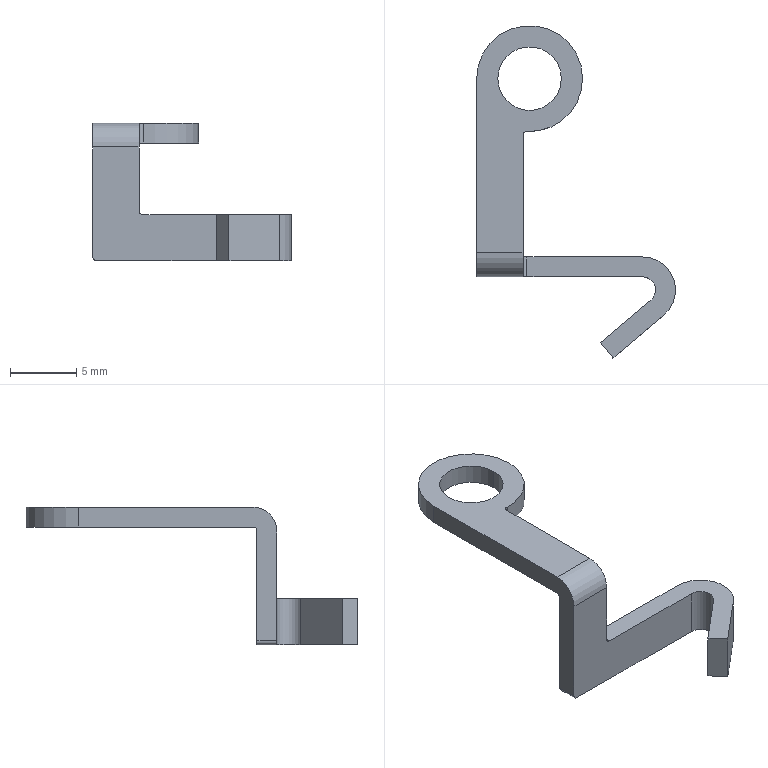Part | STEP file | TQ-DD-1105-THTerminalD1010_デフォルト | 1 solid | 22 faces | box 15.02 x 25.091 x 10.4 mm | volume 251.396 mm3 | cylinder 11 | plane 11 | commonest cylinder face diameters 0.6 x4 4.8 x2 8 x2 2 x1 3.6 x1 5 x1
STEP:
#1=CARTESIAN_POINT('',(2.4,0.,0.));
#2=VERTEX_POINT('',#1);
#3=CARTESIAN_POINT('',(-2.4,0.,0.));
#4=VERTEX_POINT('',#3);
#5=CARTESIAN_POINT('',(0.,0.,0.));
#6=DIRECTION('',(0.,0.,-1.));
#7=DIRECTION('',(1.,0.,0.));
#8=AXIS2_PLACEMENT_3D('',#5,#6,#7);
#9=CIRCLE('',#8,2.4);
#10=EDGE_CURVE('',#2,#4,#9,.T.);
#11=ORIENTED_EDGE('',*,*,#10,.T.);
#12=CARTESIAN_POINT('',(-2.4,0.,1.5));
#13=VERTEX_POINT('',#12);
#14=CARTESIAN_POINT('',(-2.4,0.,0.75));
#15=DIRECTION('',(0.,0.,1.));
#16=VECTOR('',#15,1000.);
#17=LINE('',#14,#16);
#18=EDGE_CURVE('',#4,#13,#17,.T.);
#19=ORIENTED_EDGE('',*,*,#18,.T.);
#20=CARTESIAN_POINT('',(2.4,0.,1.5));
#21=VERTEX_POINT('',#20);
#22=CARTESIAN_POINT('',(0.,0.,1.5));
#23=DIRECTION('',(0.,0.,-1.));
#24=DIRECTION('',(1.,0.,0.));
#25=AXIS2_PLACEMENT_3D('',#22,#23,#24);
#26=CIRCLE('',#25,2.4);
#27=EDGE_CURVE('',#21,#13,#26,.T.);
#28=ORIENTED_EDGE('',*,*,#27,.F.);
#29=CARTESIAN_POINT('',(2.4,0.,0.75));
#30=DIRECTION('',(0.,0.,1.));
#31=VECTOR('',#30,1000.);
#32=LINE('',#29,#31);
#33=EDGE_CURVE('',#2,#21,#32,.T.);
#34=ORIENTED_EDGE('',*,*,#33,.F.);
#35=EDGE_LOOP('',(#11,#19,#28,#34));
#36=FACE_OUTER_BOUND('',#35,.T.);
#37=CARTESIAN_POINT('',(0.,0.,0.75));
#38=DIRECTION('',(0.,0.,1.));
#39=DIRECTION('',(1.,0.,0.));
#40=AXIS2_PLACEMENT_3D('',#37,#38,#39);
#41=CYLINDRICAL_SURFACE('',#40,2.4);
#42=ADVANCED_FACE('',(#36),#41,.F.);
#43=CARTESIAN_POINT('',(-0.186,-3.996,0.));
#44=VERTEX_POINT('',#43);
#45=CARTESIAN_POINT('',(4.,0.,0.));
#46=VERTEX_POINT('',#45);
#47=CARTESIAN_POINT('',(0.,0.,0.));
#48=DIRECTION('',(0.,0.,1.));
#49=DIRECTION('',(1.,0.,0.));
#50=AXIS2_PLACEMENT_3D('',#47,#48,#49);
#51=CIRCLE('',#50,4.);
#52=EDGE_CURVE('',#44,#46,#51,.T.);
#53=ORIENTED_EDGE('',*,*,#52,.T.);
#54=CARTESIAN_POINT('',(4.,0.,1.5));
#55=VERTEX_POINT('',#54);
#56=CARTESIAN_POINT('',(4.,0.,0.75));
#57=DIRECTION('',(0.,0.,1.));
#58=VECTOR('',#57,1000.);
#59=LINE('',#56,#58);
#60=EDGE_CURVE('',#46,#55,#59,.T.);
#61=ORIENTED_EDGE('',*,*,#60,.T.);
#62=CARTESIAN_POINT('',(-0.186,-3.996,1.5));
#63=VERTEX_POINT('',#62);
#64=CARTESIAN_POINT('',(0.,0.,1.5));
#65=DIRECTION('',(0.,0.,-1.));
#66=DIRECTION('',(1.,0.,0.));
#67=AXIS2_PLACEMENT_3D('',#64,#65,#66);
#68=CIRCLE('',#67,4.);
#69=EDGE_CURVE('',#55,#63,#68,.T.);
#70=ORIENTED_EDGE('',*,*,#69,.T.);
#71=CARTESIAN_POINT('',(-0.186,-3.996,0.75));
#72=DIRECTION('',(0.,0.,-1.));
#73=VECTOR('',#72,1000.);
#74=LINE('',#71,#73);
#75=EDGE_CURVE('',#63,#44,#74,.T.);
#76=ORIENTED_EDGE('',*,*,#75,.T.);
#77=EDGE_LOOP('',(#53,#61,#70,#76));
#78=FACE_OUTER_BOUND('',#77,.T.);
#79=CARTESIAN_POINT('',(0.,0.,0.75));
#80=DIRECTION('',(0.,0.,1.));
#81=DIRECTION('',(1.,0.,0.));
#82=AXIS2_PLACEMENT_3D('',#79,#80,#81);
#83=CYLINDRICAL_SURFACE('',#82,4.);
#84=ADVANCED_FACE('',(#78),#83,.T.);
#85=ORIENTED_EDGE('',*,*,#10,.F.);
#86=CARTESIAN_POINT('',(0.,0.,0.));
#87=DIRECTION('',(0.,0.,-1.));
#88=DIRECTION('',(1.,0.,0.));
#89=AXIS2_PLACEMENT_3D('',#86,#87,#88);
#90=CIRCLE('',#89,2.4);
#91=EDGE_CURVE('',#4,#2,#90,.T.);
#92=ORIENTED_EDGE('',*,*,#91,.F.);
#93=EDGE_LOOP('',(#85,#92));
#94=FACE_BOUND('',#93,.T.);
#95=CARTESIAN_POINT('',(-4.,0.,0.));
#96=VERTEX_POINT('',#95);
#97=CARTESIAN_POINT('',(-4.,-13.162,0.));
#98=VERTEX_POINT('',#97);
#99=CARTESIAN_POINT('',(-4.,0.,0.));
#100=DIRECTION('',(0.,-1.,0.));
#101=VECTOR('',#100,1000.);
#102=LINE('',#99,#101);
#103=EDGE_CURVE('',#96,#98,#102,.T.);
#104=ORIENTED_EDGE('',*,*,#103,.F.);
#105=CARTESIAN_POINT('',(0.,0.,0.));
#106=DIRECTION('',(0.,0.,1.));
#107=DIRECTION('',(1.,0.,0.));
#108=AXIS2_PLACEMENT_3D('',#105,#106,#107);
#109=CIRCLE('',#108,4.);
#110=EDGE_CURVE('',#46,#96,#109,.T.);
#111=ORIENTED_EDGE('',*,*,#110,.F.);
#112=ORIENTED_EDGE('',*,*,#52,.F.);
#113=CARTESIAN_POINT('',(-0.5,-4.295,0.));
#114=VERTEX_POINT('',#113);
#115=CARTESIAN_POINT('',(-0.2,-4.295,0.));
#116=DIRECTION('',(0.,0.,1.));
#117=DIRECTION('',(1.,0.,0.));
#118=AXIS2_PLACEMENT_3D('',#115,#116,#117);
#119=CIRCLE('',#118,0.3);
#120=EDGE_CURVE('',#44,#114,#119,.T.);
#121=ORIENTED_EDGE('',*,*,#120,.T.);
#122=CARTESIAN_POINT('',(-0.5,-13.162,0.));
#123=VERTEX_POINT('',#122);
#124=CARTESIAN_POINT('',(-0.5,0.,0.));
#125=DIRECTION('',(0.,1.,0.));
#126=VECTOR('',#125,1000.);
#127=LINE('',#124,#126);
#128=EDGE_CURVE('',#123,#114,#127,.T.);
#129=ORIENTED_EDGE('',*,*,#128,.F.);
#130=CARTESIAN_POINT('',(0.,-13.162,0.));
#131=DIRECTION('',(1.,0.,0.));
#132=VECTOR('',#131,1000.);
#133=LINE('',#130,#132);
#134=EDGE_CURVE('',#98,#123,#133,.T.);
#135=ORIENTED_EDGE('',*,*,#134,.F.);
#136=EDGE_LOOP('',(#104,#111,#112,#121,#129,#135));
#137=FACE_OUTER_BOUND('',#136,.T.);
#138=CARTESIAN_POINT('',(0.,0.,0.));
#139=DIRECTION('',(0.,0.,1.));
#140=DIRECTION('',(1.,0.,0.));
#141=AXIS2_PLACEMENT_3D('',#138,#139,#140);
#142=PLANE('',#141);
#143=ADVANCED_FACE('',(#94,#137),#142,.F.);
#144=ORIENTED_EDGE('',*,*,#18,.F.);
#145=ORIENTED_EDGE('',*,*,#91,.T.);
#146=ORIENTED_EDGE('',*,*,#33,.T.);
#147=CARTESIAN_POINT('',(0.,0.,1.5));
#148=DIRECTION('',(0.,0.,-1.));
#149=DIRECTION('',(1.,0.,0.));
#150=AXIS2_PLACEMENT_3D('',#147,#148,#149);
#151=CIRCLE('',#150,2.4);
#152=EDGE_CURVE('',#13,#21,#151,.T.);
#153=ORIENTED_EDGE('',*,*,#152,.F.);
#154=EDGE_LOOP('',(#144,#145,#146,#153));
#155=FACE_OUTER_BOUND('',#154,.T.);
#156=CARTESIAN_POINT('',(0.,0.,0.75));
#157=DIRECTION('',(0.,0.,1.));
#158=DIRECTION('',(1.,0.,0.));
#159=AXIS2_PLACEMENT_3D('',#156,#157,#158);
#160=CYLINDRICAL_SURFACE('',#159,2.4);
#161=ADVANCED_FACE('',(#155),#160,.F.);
#162=CARTESIAN_POINT('',(-0.5,-13.462,-0.3));
#163=VERTEX_POINT('',#162);
#164=CARTESIAN_POINT('',(-0.5,-13.162,-0.3));
#165=DIRECTION('',(-1.,0.,0.));
#166=DIRECTION('',(0.,0.,-1.));
#167=AXIS2_PLACEMENT_3D('',#164,#165,#166);
#168=CIRCLE('',#167,0.3);
#169=EDGE_CURVE('',#163,#123,#168,.T.);
#170=ORIENTED_EDGE('',*,*,#169,.F.);
#171=CARTESIAN_POINT('',(-4.,-13.462,-0.3));
#172=VERTEX_POINT('',#171);
#173=CARTESIAN_POINT('',(0.,-13.462,-0.3));
#174=DIRECTION('',(1.,0.,0.));
#175=VECTOR('',#174,1000.);
#176=LINE('',#173,#175);
#177=EDGE_CURVE('',#172,#163,#176,.T.);
#178=ORIENTED_EDGE('',*,*,#177,.F.);
#179=CARTESIAN_POINT('',(-4.,-13.162,-0.3));
#180=DIRECTION('',(1.,0.,0.));
#181=DIRECTION('',(0.,0.,-1.));
#182=AXIS2_PLACEMENT_3D('',#179,#180,#181);
#183=CIRCLE('',#182,0.3);
#184=EDGE_CURVE('',#98,#172,#183,.T.);
#185=ORIENTED_EDGE('',*,*,#184,.F.);
#186=ORIENTED_EDGE('',*,*,#134,.T.);
#187=EDGE_LOOP('',(#170,#178,#185,#186));
#188=FACE_OUTER_BOUND('',#187,.T.);
#189=CARTESIAN_POINT('',(0.,-13.162,-0.3));
#190=DIRECTION('',(1.,0.,0.));
#191=DIRECTION('',(0.,0.,-1.));
#192=AXIS2_PLACEMENT_3D('',#189,#190,#191);
#193=CYLINDRICAL_SURFACE('',#192,0.3);
#194=ADVANCED_FACE('',(#188),#193,.F.);
#195=CARTESIAN_POINT('',(-4.,-13.462,-8.6));
#196=VERTEX_POINT('',#195);
#197=CARTESIAN_POINT('',(-4.,-13.462,0.));
#198=DIRECTION('',(0.,0.,-1.));
#199=VECTOR('',#198,1000.);
#200=LINE('',#197,#199);
#201=EDGE_CURVE('',#172,#196,#200,.T.);
#202=ORIENTED_EDGE('',*,*,#201,.T.);
#203=CARTESIAN_POINT('',(-4.,-14.962,-8.6));
#204=VERTEX_POINT('',#203);
#205=CARTESIAN_POINT('',(-4.,0.,-8.6));
#206=DIRECTION('',(0.,-1.,0.));
#207=VECTOR('',#206,1000.);
#208=LINE('',#205,#207);
#209=EDGE_CURVE('',#196,#204,#208,.T.);
#210=ORIENTED_EDGE('',*,*,#209,.T.);
#211=CARTESIAN_POINT('',(-4.,-14.962,-0.3));
#212=VERTEX_POINT('',#211);
#213=CARTESIAN_POINT('',(-4.,-14.962,0.));
#214=DIRECTION('',(0.,0.,1.));
#215=VECTOR('',#214,1000.);
#216=LINE('',#213,#215);
#217=EDGE_CURVE('',#204,#212,#216,.T.);
#218=ORIENTED_EDGE('',*,*,#217,.T.);
#219=CARTESIAN_POINT('',(-4.,-13.162,1.5));
#220=VERTEX_POINT('',#219);
#221=CARTESIAN_POINT('',(-4.,-13.162,-0.3));
#222=DIRECTION('',(-1.,0.,0.));
#223=DIRECTION('',(0.,0.,1.));
#224=AXIS2_PLACEMENT_3D('',#221,#222,#223);
#225=CIRCLE('',#224,1.8);
#226=EDGE_CURVE('',#212,#220,#225,.T.);
#227=ORIENTED_EDGE('',*,*,#226,.T.);
#228=CARTESIAN_POINT('',(-4.,0.,1.5));
#229=VERTEX_POINT('',#228);
#230=CARTESIAN_POINT('',(-4.,0.,1.5));
#231=DIRECTION('',(0.,1.,0.));
#232=VECTOR('',#231,1000.);
#233=LINE('',#230,#232);
#234=EDGE_CURVE('',#220,#229,#233,.T.);
#235=ORIENTED_EDGE('',*,*,#234,.T.);
#236=CARTESIAN_POINT('',(-4.,0.,0.));
#237=DIRECTION('',(0.,0.,-1.));
#238=VECTOR('',#237,1000.);
#239=LINE('',#236,#238);
#240=EDGE_CURVE('',#229,#96,#239,.T.);
#241=ORIENTED_EDGE('',*,*,#240,.T.);
#242=ORIENTED_EDGE('',*,*,#103,.T.);
#243=ORIENTED_EDGE('',*,*,#184,.T.);
#244=EDGE_LOOP('',(#202,#210,#218,#227,#235,#241,#242,#243));
#245=FACE_OUTER_BOUND('',#244,.T.);
#246=CARTESIAN_POINT('',(-4.,0.,0.));
#247=DIRECTION('',(-1.,0.,0.));
#248=DIRECTION('',(0.,0.,1.));
#249=AXIS2_PLACEMENT_3D('',#246,#247,#248);
#250=PLANE('',#249);
#251=ADVANCED_FACE('',(#245),#250,.T.);
#252=ORIENTED_EDGE('',*,*,#60,.F.);
#253=ORIENTED_EDGE('',*,*,#110,.T.);
#254=ORIENTED_EDGE('',*,*,#240,.F.);
#255=CARTESIAN_POINT('',(0.,0.,1.5));
#256=DIRECTION('',(0.,0.,-1.));
#257=DIRECTION('',(1.,0.,0.));
#258=AXIS2_PLACEMENT_3D('',#255,#256,#257);
#259=CIRCLE('',#258,4.);
#260=EDGE_CURVE('',#229,#55,#259,.T.);
#261=ORIENTED_EDGE('',*,*,#260,.T.);
#262=EDGE_LOOP('',(#252,#253,#254,#261));
#263=FACE_OUTER_BOUND('',#262,.T.);
#264=CARTESIAN_POINT('',(0.,0.,0.75));
#265=DIRECTION('',(0.,0.,1.));
#266=DIRECTION('',(1.,0.,0.));
#267=AXIS2_PLACEMENT_3D('',#264,#265,#266);
#268=CYLINDRICAL_SURFACE('',#267,4.);
#269=ADVANCED_FACE('',(#263),#268,.T.);
#270=CARTESIAN_POINT('',(-0.5,-14.962,-0.3));
#271=VERTEX_POINT('',#270);
#272=CARTESIAN_POINT('',(-0.5,-14.962,-5.1));
#273=VERTEX_POINT('',#272);
#274=CARTESIAN_POINT('',(-0.5,-14.962,0.));
#275=DIRECTION('',(0.,0.,-1.));
#276=VECTOR('',#275,1000.);
#277=LINE('',#274,#276);
#278=EDGE_CURVE('',#271,#273,#277,.T.);
#279=ORIENTED_EDGE('',*,*,#278,.T.);
#280=CARTESIAN_POINT('',(-0.5,-13.462,-5.1));
#281=VERTEX_POINT('',#280);
#282=CARTESIAN_POINT('',(-0.5,-14.962,-5.1));
#283=DIRECTION('',(0.,1.,0.));
#284=VECTOR('',#283,1000.);
#285=LINE('',#282,#284);
#286=EDGE_CURVE('',#273,#281,#285,.T.);
#287=ORIENTED_EDGE('',*,*,#286,.T.);
#288=CARTESIAN_POINT('',(-0.5,-13.462,0.));
#289=DIRECTION('',(0.,0.,1.));
#290=VECTOR('',#289,1000.);
#291=LINE('',#288,#290);
#292=EDGE_CURVE('',#281,#163,#291,.T.);
#293=ORIENTED_EDGE('',*,*,#292,.T.);
#294=ORIENTED_EDGE('',*,*,#169,.T.);
#295=ORIENTED_EDGE('',*,*,#128,.T.);
#296=CARTESIAN_POINT('',(-0.5,-4.295,1.5));
#297=VERTEX_POINT('',#296);
#298=CARTESIAN_POINT('',(-0.5,-4.295,0.));
#299=DIRECTION('',(0.,0.,1.));
#300=VECTOR('',#299,1000.);
#301=LINE('',#298,#300);
#302=EDGE_CURVE('',#114,#297,#301,.T.);
#303=ORIENTED_EDGE('',*,*,#302,.T.);
#304=CARTESIAN_POINT('',(-0.5,-13.162,1.5));
#305=VERTEX_POINT('',#304);
#306=CARTESIAN_POINT('',(-0.5,-14.962,1.5));
#307=DIRECTION('',(0.,-1.,0.));
#308=VECTOR('',#307,1000.);
#309=LINE('',#306,#308);
#310=EDGE_CURVE('',#297,#305,#309,.T.);
#311=ORIENTED_EDGE('',*,*,#310,.T.);
#312=CARTESIAN_POINT('',(-0.5,-13.162,-0.3));
#313=DIRECTION('',(1.,0.,0.));
#314=DIRECTION('',(0.,0.,1.));
#315=AXIS2_PLACEMENT_3D('',#312,#313,#314);
#316=CIRCLE('',#315,1.8);
#317=EDGE_CURVE('',#305,#271,#316,.T.);
#318=ORIENTED_EDGE('',*,*,#317,.T.);
#319=EDGE_LOOP('',(#279,#287,#293,#294,#295,#303,#311,#318));
#320=FACE_OUTER_BOUND('',#319,.T.);
#321=CARTESIAN_POINT('',(-0.5,-14.962,0.));
#322=DIRECTION('',(1.,0.,0.));
#323=DIRECTION('',(0.,0.,-1.));
#324=AXIS2_PLACEMENT_3D('',#321,#322,#323);
#325=PLANE('',#324);
#326=ADVANCED_FACE('',(#320),#325,.T.);
#327=ORIENTED_EDGE('',*,*,#27,.T.);
#328=ORIENTED_EDGE('',*,*,#152,.T.);
#329=EDGE_LOOP('',(#327,#328));
#330=FACE_BOUND('',#329,.T.);
#331=ORIENTED_EDGE('',*,*,#234,.F.);
#332=CARTESIAN_POINT('',(0.,-13.162,1.5));
#333=DIRECTION('',(1.,0.,0.));
#334=VECTOR('',#333,1000.);
#335=LINE('',#332,#334);
#336=EDGE_CURVE('',#220,#305,#335,.T.);
#337=ORIENTED_EDGE('',*,*,#336,.T.);
#338=ORIENTED_EDGE('',*,*,#310,.F.);
#339=CARTESIAN_POINT('',(-0.2,-4.295,1.5));
#340=DIRECTION('',(0.,0.,-1.));
#341=DIRECTION('',(1.,0.,0.));
#342=AXIS2_PLACEMENT_3D('',#339,#340,#341);
#343=CIRCLE('',#342,0.3);
#344=EDGE_CURVE('',#297,#63,#343,.T.);
#345=ORIENTED_EDGE('',*,*,#344,.T.);
#346=ORIENTED_EDGE('',*,*,#69,.F.);
#347=ORIENTED_EDGE('',*,*,#260,.F.);
#348=EDGE_LOOP('',(#331,#337,#338,#345,#346,#347));
#349=FACE_OUTER_BOUND('',#348,.T.);
#350=CARTESIAN_POINT('',(0.,0.,1.5));
#351=DIRECTION('',(0.,0.,1.));
#352=DIRECTION('',(1.,0.,0.));
#353=AXIS2_PLACEMENT_3D('',#350,#351,#352);
#354=PLANE('',#353);
#355=ADVANCED_FACE('',(#330,#349),#354,.T.);
#356=ORIENTED_EDGE('',*,*,#201,.F.);
#357=ORIENTED_EDGE('',*,*,#177,.T.);
#358=ORIENTED_EDGE('',*,*,#292,.F.);
#359=CARTESIAN_POINT('',(-0.2,-13.462,-5.4));
#360=VERTEX_POINT('',#359);
#361=CARTESIAN_POINT('',(-0.2,-13.462,-5.1));
#362=DIRECTION('',(0.,1.,0.));
#363=DIRECTION('',(0.,0.,1.));
#364=AXIS2_PLACEMENT_3D('',#361,#362,#363);
#365=CIRCLE('',#364,0.3);
#366=EDGE_CURVE('',#360,#281,#365,.T.);
#367=ORIENTED_EDGE('',*,*,#366,.F.);
#368=CARTESIAN_POINT('',(8.52,-13.462,-5.4));
#369=VERTEX_POINT('',#368);
#370=CARTESIAN_POINT('',(-0.5,-13.462,-5.4));
#371=DIRECTION('',(-1.,0.,0.));
#372=VECTOR('',#371,1000.);
#373=LINE('',#370,#372);
#374=EDGE_CURVE('',#369,#360,#373,.T.);
#375=ORIENTED_EDGE('',*,*,#374,.F.);
#376=CARTESIAN_POINT('',(8.52,-13.462,-8.9));
#377=VERTEX_POINT('',#376);
#378=CARTESIAN_POINT('',(8.52,-13.462,-8.9));
#379=DIRECTION('',(0.,0.,1.));
#380=VECTOR('',#379,1000.);
#381=LINE('',#378,#380);
#382=EDGE_CURVE('',#377,#369,#381,.T.);
#383=ORIENTED_EDGE('',*,*,#382,.F.);
#384=CARTESIAN_POINT('',(-3.7,-13.462,-8.9));
#385=VERTEX_POINT('',#384);
#386=CARTESIAN_POINT('',(-0.5,-13.462,-8.9));
#387=DIRECTION('',(1.,0.,0.));
#388=VECTOR('',#387,1000.);
#389=LINE('',#386,#388);
#390=EDGE_CURVE('',#385,#377,#389,.T.);
#391=ORIENTED_EDGE('',*,*,#390,.F.);
#392=CARTESIAN_POINT('',(-3.7,-13.462,-8.6));
#393=DIRECTION('',(0.,-1.,0.));
#394=DIRECTION('',(0.,0.,1.));
#395=AXIS2_PLACEMENT_3D('',#392,#393,#394);
#396=CIRCLE('',#395,0.3);
#397=EDGE_CURVE('',#196,#385,#396,.T.);
#398=ORIENTED_EDGE('',*,*,#397,.F.);
#399=EDGE_LOOP('',(#356,#357,#358,#367,#375,#383,#391,#398));
#400=FACE_OUTER_BOUND('',#399,.T.);
#401=CARTESIAN_POINT('',(-0.5,-13.462,-8.9));
#402=DIRECTION('',(0.,-1.,0.));
#403=DIRECTION('',(0.,0.,-1.));
#404=AXIS2_PLACEMENT_3D('',#401,#402,#403);
#405=PLANE('',#404);
#406=ADVANCED_FACE('',(#400),#405,.F.);
#407=CARTESIAN_POINT('',(-3.7,-14.962,-8.9));
#408=VERTEX_POINT('',#407);
#409=CARTESIAN_POINT('',(-3.7,-14.962,-8.6));
#410=DIRECTION('',(0.,1.,0.));
#411=DIRECTION('',(0.,0.,1.));
#412=AXIS2_PLACEMENT_3D('',#409,#410,#411);
#413=CIRCLE('',#412,0.3);
#414=EDGE_CURVE('',#408,#204,#413,.T.);
#415=ORIENTED_EDGE('',*,*,#414,.T.);
#416=ORIENTED_EDGE('',*,*,#209,.F.);
#417=ORIENTED_EDGE('',*,*,#397,.T.);
#418=CARTESIAN_POINT('',(-3.7,-9.812,-8.9));
#419=DIRECTION('',(0.,-1.,0.));
#420=VECTOR('',#419,1000.);
#421=LINE('',#418,#420);
#422=EDGE_CURVE('',#385,#408,#421,.T.);
#423=ORIENTED_EDGE('',*,*,#422,.T.);
#424=EDGE_LOOP('',(#415,#416,#417,#423));
#425=FACE_OUTER_BOUND('',#424,.T.);
#426=CARTESIAN_POINT('',(-3.7,-9.812,-8.6));
#427=DIRECTION('',(0.,1.,0.));
#428=DIRECTION('',(0.,0.,1.));
#429=AXIS2_PLACEMENT_3D('',#426,#427,#428);
#430=CYLINDRICAL_SURFACE('',#429,0.3);
#431=ADVANCED_FACE('',(#425),#430,.T.);
#432=ORIENTED_EDGE('',*,*,#317,.F.);
#433=ORIENTED_EDGE('',*,*,#336,.F.);
#434=ORIENTED_EDGE('',*,*,#226,.F.);
#435=CARTESIAN_POINT('',(0.,-14.962,-0.3));
#436=DIRECTION('',(1.,0.,0.));
#437=VECTOR('',#436,1000.);
#438=LINE('',#435,#437);
#439=EDGE_CURVE('',#212,#271,#438,.T.);
#440=ORIENTED_EDGE('',*,*,#439,.T.);
#441=EDGE_LOOP('',(#432,#433,#434,#440));
#442=FACE_OUTER_BOUND('',#441,.T.);
#443=CARTESIAN_POINT('',(0.,-13.162,-0.3));
#444=DIRECTION('',(-1.,0.,0.));
#445=DIRECTION('',(0.,0.,1.));
#446=AXIS2_PLACEMENT_3D('',#443,#444,#445);
#447=CYLINDRICAL_SURFACE('',#446,1.8);
#448=ADVANCED_FACE('',(#442),#447,.T.);
#449=CARTESIAN_POINT('',(8.52,-14.962,-8.9));
#450=VERTEX_POINT('',#449);
#451=CARTESIAN_POINT('',(-0.5,-14.962,-8.9));
#452=DIRECTION('',(-1.,0.,0.));
#453=VECTOR('',#452,1000.);
#454=LINE('',#451,#453);
#455=EDGE_CURVE('',#450,#408,#454,.T.);
#456=ORIENTED_EDGE('',*,*,#455,.F.);
#457=CARTESIAN_POINT('',(8.52,-14.962,-5.4));
#458=VERTEX_POINT('',#457);
#459=CARTESIAN_POINT('',(8.52,-14.962,0.));
#460=DIRECTION('',(0.,0.,-1.));
#461=VECTOR('',#460,1000.);
#462=LINE('',#459,#461);
#463=EDGE_CURVE('',#458,#450,#462,.T.);
#464=ORIENTED_EDGE('',*,*,#463,.F.);
#465=CARTESIAN_POINT('',(-0.2,-14.962,-5.4));
#466=VERTEX_POINT('',#465);
#467=CARTESIAN_POINT('',(-0.5,-14.962,-5.4));
#468=DIRECTION('',(1.,0.,0.));
#469=VECTOR('',#468,1000.);
#470=LINE('',#467,#469);
#471=EDGE_CURVE('',#466,#458,#470,.T.);
#472=ORIENTED_EDGE('',*,*,#471,.F.);
#473=CARTESIAN_POINT('',(-0.2,-14.962,-5.1));
#474=DIRECTION('',(0.,-1.,0.));
#475=DIRECTION('',(0.,0.,1.));
#476=AXIS2_PLACEMENT_3D('',#473,#474,#475);
#477=CIRCLE('',#476,0.3);
#478=EDGE_CURVE('',#273,#466,#477,.T.);
#479=ORIENTED_EDGE('',*,*,#478,.F.);
#480=ORIENTED_EDGE('',*,*,#278,.F.);
#481=ORIENTED_EDGE('',*,*,#439,.F.);
#482=ORIENTED_EDGE('',*,*,#217,.F.);
#483=ORIENTED_EDGE('',*,*,#414,.F.);
#484=EDGE_LOOP('',(#456,#464,#472,#479,#480,#481,#482,#483));
#485=FACE_OUTER_BOUND('',#484,.T.);
#486=CARTESIAN_POINT('',(-0.5,-14.962,0.));
#487=DIRECTION('',(0.,1.,0.));
#488=DIRECTION('',(0.,0.,1.));
#489=AXIS2_PLACEMENT_3D('',#486,#487,#488);
#490=PLANE('',#489);
#491=ADVANCED_FACE('',(#485),#490,.F.);
#492=ORIENTED_EDGE('',*,*,#120,.F.);
#493=ORIENTED_EDGE('',*,*,#75,.F.);
#494=ORIENTED_EDGE('',*,*,#344,.F.);
#495=ORIENTED_EDGE('',*,*,#302,.F.);
#496=EDGE_LOOP('',(#492,#493,#494,#495));
#497=FACE_OUTER_BOUND('',#496,.T.);
#498=CARTESIAN_POINT('',(-0.2,-4.295,0.75));
#499=DIRECTION('',(0.,0.,1.));
#500=DIRECTION('',(1.,0.,0.));
#501=AXIS2_PLACEMENT_3D('',#498,#499,#500);
#502=CYLINDRICAL_SURFACE('',#501,0.3);
#503=ADVANCED_FACE('',(#497),#502,.F.);
#504=ORIENTED_EDGE('',*,*,#366,.T.);
#505=ORIENTED_EDGE('',*,*,#286,.F.);
#506=ORIENTED_EDGE('',*,*,#478,.T.);
#507=CARTESIAN_POINT('',(-0.2,-12.389,-5.4));
#508=DIRECTION('',(0.,-1.,0.));
#509=VECTOR('',#508,1000.);
#510=LINE('',#507,#509);
#511=EDGE_CURVE('',#360,#466,#510,.T.);
#512=ORIENTED_EDGE('',*,*,#511,.F.);
#513=EDGE_LOOP('',(#504,#505,#506,#512));
#514=FACE_OUTER_BOUND('',#513,.T.);
#515=CARTESIAN_POINT('',(-0.2,-12.389,-5.1));
#516=DIRECTION('',(0.,1.,0.));
#517=DIRECTION('',(0.,0.,1.));
#518=AXIS2_PLACEMENT_3D('',#515,#516,#517);
#519=CYLINDRICAL_SURFACE('',#518,0.3);
#520=ADVANCED_FACE('',(#514),#519,.F.);
#521=ORIENTED_EDGE('',*,*,#374,.T.);
#522=ORIENTED_EDGE('',*,*,#511,.T.);
#523=ORIENTED_EDGE('',*,*,#471,.T.);
#524=CARTESIAN_POINT('',(9.163,-16.728,-5.4));
#525=VERTEX_POINT('',#524);
#526=CARTESIAN_POINT('',(8.52,-15.962,-5.4));
#527=DIRECTION('',(0.,0.,-1.));
#528=DIRECTION('',(0.,-1.,0.));
#529=AXIS2_PLACEMENT_3D('',#526,#527,#528);
#530=CIRCLE('',#529,1.);
#531=EDGE_CURVE('',#458,#525,#530,.T.);
#532=ORIENTED_EDGE('',*,*,#531,.T.);
#533=CARTESIAN_POINT('',(5.333,-19.942,-5.4));
#534=VERTEX_POINT('',#533);
#535=CARTESIAN_POINT('',(9.163,-16.728,-5.4));
#536=DIRECTION('',(-0.766,-0.6428,0.));
#537=VECTOR('',#536,1000.);
#538=LINE('',#535,#537);
#539=EDGE_CURVE('',#525,#534,#538,.T.);
#540=ORIENTED_EDGE('',*,*,#539,.T.);
#541=CARTESIAN_POINT('',(6.297,-21.091,-5.4));
#542=VERTEX_POINT('',#541);
#543=CARTESIAN_POINT('',(5.333,-19.942,-5.4));
#544=DIRECTION('',(-0.6428,0.766,0.));
#545=VECTOR('',#544,1000.);
#546=LINE('',#543,#545);
#547=EDGE_CURVE('',#542,#534,#546,.T.);
#548=ORIENTED_EDGE('',*,*,#547,.F.);
#549=CARTESIAN_POINT('',(10.127,-17.877,-5.4));
#550=VERTEX_POINT('',#549);
#551=CARTESIAN_POINT('',(6.297,-21.091,-5.4));
#552=DIRECTION('',(0.766,0.6428,0.));
#553=VECTOR('',#552,1000.);
#554=LINE('',#551,#553);
#555=EDGE_CURVE('',#542,#550,#554,.T.);
#556=ORIENTED_EDGE('',*,*,#555,.T.);
#557=CARTESIAN_POINT('',(8.52,-15.962,-5.4));
#558=DIRECTION('',(0.,0.,1.));
#559=DIRECTION('',(0.,-1.,0.));
#560=AXIS2_PLACEMENT_3D('',#557,#558,#559);
#561=CIRCLE('',#560,2.5);
#562=EDGE_CURVE('',#550,#369,#561,.T.);
#563=ORIENTED_EDGE('',*,*,#562,.T.);
#564=EDGE_LOOP('',(#521,#522,#523,#532,#540,#548,#556,#563));
#565=FACE_OUTER_BOUND('',#564,.T.);
#566=CARTESIAN_POINT('',(0.,0.,-5.4));
#567=DIRECTION('',(0.,0.,1.));
#568=DIRECTION('',(0.,-1.,0.));
#569=AXIS2_PLACEMENT_3D('',#566,#567,#568);
#570=PLANE('',#569);
#571=ADVANCED_FACE('',(#565),#570,.T.);
#572=ORIENTED_EDGE('',*,*,#382,.T.);
#573=ORIENTED_EDGE('',*,*,#562,.F.);
#574=CARTESIAN_POINT('',(10.127,-17.877,-8.9));
#575=VERTEX_POINT('',#574);
#576=CARTESIAN_POINT('',(10.127,-17.877,-7.15));
#577=DIRECTION('',(0.,0.,-1.));
#578=VECTOR('',#577,1000.);
#579=LINE('',#576,#578);
#580=EDGE_CURVE('',#550,#575,#579,.T.);
#581=ORIENTED_EDGE('',*,*,#580,.T.);
#582=CARTESIAN_POINT('',(8.52,-15.962,-8.9));
#583=DIRECTION('',(0.,0.,1.));
#584=DIRECTION('',(0.,-1.,0.));
#585=AXIS2_PLACEMENT_3D('',#582,#583,#584);
#586=CIRCLE('',#585,2.5);
#587=EDGE_CURVE('',#575,#377,#586,.T.);
#588=ORIENTED_EDGE('',*,*,#587,.T.);
#589=EDGE_LOOP('',(#572,#573,#581,#588));
#590=FACE_OUTER_BOUND('',#589,.T.);
#591=CARTESIAN_POINT('',(8.52,-15.962,-7.15));
#592=DIRECTION('',(0.,0.,1.));
#593=DIRECTION('',(0.,-1.,0.));
#594=AXIS2_PLACEMENT_3D('',#591,#592,#593);
#595=CYLINDRICAL_SURFACE('',#594,2.5);
#596=ADVANCED_FACE('',(#590),#595,.T.);
#597=ORIENTED_EDGE('',*,*,#455,.T.);
#598=ORIENTED_EDGE('',*,*,#422,.F.);
#599=ORIENTED_EDGE('',*,*,#390,.T.);
#600=ORIENTED_EDGE('',*,*,#587,.F.);
#601=CARTESIAN_POINT('',(6.297,-21.091,-8.9));
#602=VERTEX_POINT('',#601);
#603=CARTESIAN_POINT('',(10.127,-17.877,-8.9));
#604=DIRECTION('',(-0.766,-0.6428,0.));
#605=VECTOR('',#604,1000.);
#606=LINE('',#603,#605);
#607=EDGE_CURVE('',#575,#602,#606,.T.);
#608=ORIENTED_EDGE('',*,*,#607,.T.);
#609=CARTESIAN_POINT('',(5.333,-19.942,-8.9));
#610=VERTEX_POINT('',#609);
#611=CARTESIAN_POINT('',(5.333,-19.942,-8.9));
#612=DIRECTION('',(0.6428,-0.766,0.));
#613=VECTOR('',#612,1000.);
#614=LINE('',#611,#613);
#615=EDGE_CURVE('',#610,#602,#614,.T.);
#616=ORIENTED_EDGE('',*,*,#615,.F.);
#617=CARTESIAN_POINT('',(9.163,-16.728,-8.9));
#618=VERTEX_POINT('',#617);
#619=CARTESIAN_POINT('',(5.333,-19.942,-8.9));
#620=DIRECTION('',(0.766,0.6428,0.));
#621=VECTOR('',#620,1000.);
#622=LINE('',#619,#621);
#623=EDGE_CURVE('',#610,#618,#622,.T.);
#624=ORIENTED_EDGE('',*,*,#623,.T.);
#625=CARTESIAN_POINT('',(8.52,-15.962,-8.9));
#626=DIRECTION('',(0.,0.,1.));
#627=DIRECTION('',(0.,-1.,0.));
#628=AXIS2_PLACEMENT_3D('',#625,#626,#627);
#629=CIRCLE('',#628,1.);
#630=EDGE_CURVE('',#618,#450,#629,.T.);
#631=ORIENTED_EDGE('',*,*,#630,.T.);
#632=EDGE_LOOP('',(#597,#598,#599,#600,#608,#616,#624,#631));
#633=FACE_OUTER_BOUND('',#632,.T.);
#634=CARTESIAN_POINT('',(-0.5,-13.462,-8.9));
#635=DIRECTION('',(0.,0.,-1.));
#636=DIRECTION('',(0.,1.,0.));
#637=AXIS2_PLACEMENT_3D('',#634,#635,#636);
#638=PLANE('',#637);
#639=ADVANCED_FACE('',(#633),#638,.T.);
#640=ORIENTED_EDGE('',*,*,#630,.F.);
#641=CARTESIAN_POINT('',(9.163,-16.728,-7.15));
#642=DIRECTION('',(0.,0.,-1.));
#643=VECTOR('',#642,1000.);
#644=LINE('',#641,#643);
#645=EDGE_CURVE('',#525,#618,#644,.T.);
#646=ORIENTED_EDGE('',*,*,#645,.F.);
#647=ORIENTED_EDGE('',*,*,#531,.F.);
#648=ORIENTED_EDGE('',*,*,#463,.T.);
#649=EDGE_LOOP('',(#640,#646,#647,#648));
#650=FACE_OUTER_BOUND('',#649,.T.);
#651=CARTESIAN_POINT('',(8.52,-15.962,-7.15));
#652=DIRECTION('',(0.,0.,1.));
#653=DIRECTION('',(0.,-1.,0.));
#654=AXIS2_PLACEMENT_3D('',#651,#652,#653);
#655=CYLINDRICAL_SURFACE('',#654,1.);
#656=ADVANCED_FACE('',(#650),#655,.F.);
#657=ORIENTED_EDGE('',*,*,#580,.F.);
#658=ORIENTED_EDGE('',*,*,#555,.F.);
#659=CARTESIAN_POINT('',(6.297,-21.091,-8.9));
#660=DIRECTION('',(0.,0.,-1.));
#661=VECTOR('',#660,1000.);
#662=LINE('',#659,#661);
#663=EDGE_CURVE('',#542,#602,#662,.T.);
#664=ORIENTED_EDGE('',*,*,#663,.T.);
#665=ORIENTED_EDGE('',*,*,#607,.F.);
#666=EDGE_LOOP('',(#657,#658,#664,#665));
#667=FACE_OUTER_BOUND('',#666,.T.);
#668=CARTESIAN_POINT('',(6.297,-21.091,-8.9));
#669=DIRECTION('',(0.6428,-0.766,0.));
#670=DIRECTION('',(0.766,0.6428,0.));
#671=AXIS2_PLACEMENT_3D('',#668,#669,#670);
#672=PLANE('',#671);
#673=ADVANCED_FACE('',(#667),#672,.T.);
#674=ORIENTED_EDGE('',*,*,#623,.F.);
#675=CARTESIAN_POINT('',(5.333,-19.942,-8.9));
#676=DIRECTION('',(0.,0.,-1.));
#677=VECTOR('',#676,1000.);
#678=LINE('',#675,#677);
#679=EDGE_CURVE('',#534,#610,#678,.T.);
#680=ORIENTED_EDGE('',*,*,#679,.F.);
#681=ORIENTED_EDGE('',*,*,#539,.F.);
#682=ORIENTED_EDGE('',*,*,#645,.T.);
#683=EDGE_LOOP('',(#674,#680,#681,#682));
#684=FACE_OUTER_BOUND('',#683,.T.);
#685=CARTESIAN_POINT('',(5.333,-19.942,-8.9));
#686=DIRECTION('',(0.6428,-0.766,0.));
#687=DIRECTION('',(0.766,0.6428,0.));
#688=AXIS2_PLACEMENT_3D('',#685,#686,#687);
#689=PLANE('',#688);
#690=ADVANCED_FACE('',(#684),#689,.F.);
#691=ORIENTED_EDGE('',*,*,#663,.F.);
#692=ORIENTED_EDGE('',*,*,#547,.T.);
#693=ORIENTED_EDGE('',*,*,#679,.T.);
#694=ORIENTED_EDGE('',*,*,#615,.T.);
#695=EDGE_LOOP('',(#691,#692,#693,#694));
#696=FACE_OUTER_BOUND('',#695,.T.);
#697=CARTESIAN_POINT('',(5.333,-19.942,-8.9));
#698=DIRECTION('',(-0.766,-0.6428,0.));
#699=DIRECTION('',(0.6428,-0.766,0.));
#700=AXIS2_PLACEMENT_3D('',#697,#698,#699);
#701=PLANE('',#700);
#702=ADVANCED_FACE('',(#696),#701,.T.);
#703=CLOSED_SHELL('',(#42,#84,#143,#161,#194,#251,#269,#326,#355,#406,#431,#448,#491,#503,#520,#571,#596,#639,#656,#673,#690,#702));
#704=MANIFOLD_SOLID_BREP('',#703);
#705=CARTESIAN_POINT('',(0.,0.,0.));
#706=DIRECTION('',(0.,0.,1.));
#707=DIRECTION('',(1.,0.,0.));
#708=AXIS2_PLACEMENT_3D('',#705,#706,#707);
#709=(LENGTH_UNIT()NAMED_UNIT(*)SI_UNIT(.MILLI.,.METRE.));
#710=UNCERTAINTY_MEASURE_WITH_UNIT(LENGTH_MEASURE(0.00001),#709,'','');
#711=(NAMED_UNIT(*)PLANE_ANGLE_UNIT()SI_UNIT($,.RADIAN.));
#712=(NAMED_UNIT(*)SI_UNIT($,.STERADIAN.)SOLID_ANGLE_UNIT());
#713=(GEOMETRIC_REPRESENTATION_CONTEXT(3)GLOBAL_UNCERTAINTY_ASSIGNED_CONTEXT((#710))GLOBAL_UNIT_ASSIGNED_CONTEXT((#709,#711,#712))REPRESENTATION_CONTEXT('',''));
#714=ADVANCED_BREP_SHAPE_REPRESENTATION('',(#704,#708),#713);